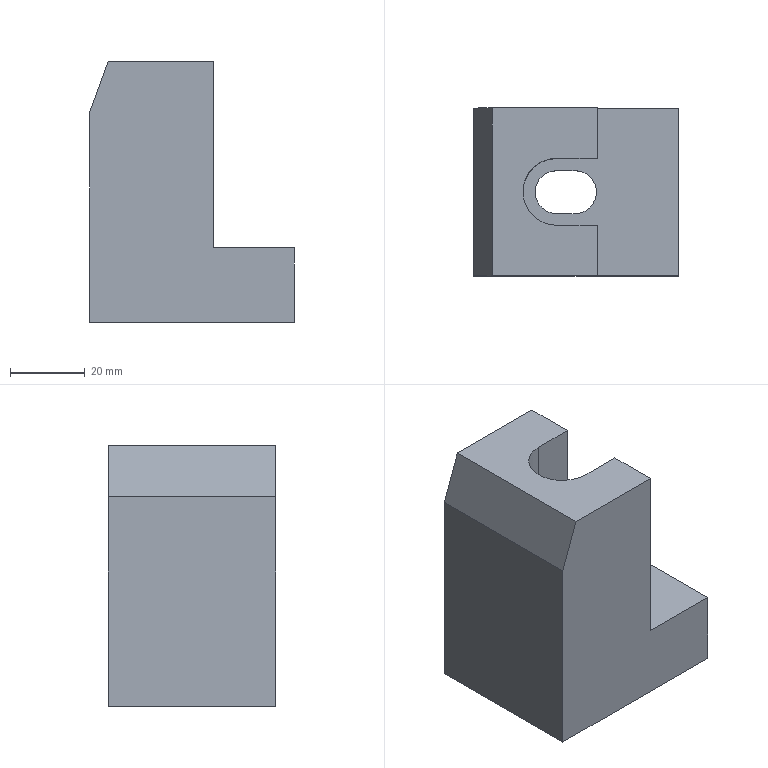Part | STEP file | lll_id5026_x_t | 1 solid | 17 faces | box 55 x 45 x 70 mm | volume 103267 mm3 | plane 14 | cylinder 3 | commonest cylinder face diameters 11.509 x2 18.008 x1
STEP:
#1=CARTESIAN_POINT('',(2858.213,-91.496,0.));
#2=VERTEX_POINT('',#1);
#3=CARTESIAN_POINT('',(2858.213,-78.,0.));
#4=VERTEX_POINT('',#3);
#5=CARTESIAN_POINT('',(2858.213,-123.,0.));
#6=DIRECTION('',(0.,1.,0.));
#7=VECTOR('',#6,1.);
#8=LINE('',#5,#7);
#9=EDGE_CURVE('',#2,#4,#8,.T.);
#10=ORIENTED_EDGE('',*,*,#9,.T.);
#11=CARTESIAN_POINT('',(2858.213,-78.,50.));
#12=VERTEX_POINT('',#11);
#13=CARTESIAN_POINT('',(2858.213,-78.,25.));
#14=DIRECTION('',(0.,0.,-1.));
#15=VECTOR('',#14,1.);
#16=LINE('',#13,#15);
#17=EDGE_CURVE('',#12,#4,#16,.T.);
#18=ORIENTED_EDGE('',*,*,#17,.F.);
#19=CARTESIAN_POINT('',(2858.213,-91.496,50.));
#20=VERTEX_POINT('',#19);
#21=CARTESIAN_POINT('',(2858.213,-173.,50.));
#22=DIRECTION('',(0.,1.,0.));
#23=VECTOR('',#22,1.);
#24=LINE('',#21,#23);
#25=EDGE_CURVE('',#20,#12,#24,.T.);
#26=ORIENTED_EDGE('',*,*,#25,.F.);
#27=CARTESIAN_POINT('',(2858.213,-91.496,0.));
#28=DIRECTION('',(0.,0.,1.));
#29=VECTOR('',#28,1.);
#30=LINE('',#27,#29);
#31=EDGE_CURVE('',#2,#20,#30,.T.);
#32=ORIENTED_EDGE('',*,*,#31,.F.);
#33=EDGE_LOOP('',(#10,#18,#26,#32));
#34=FACE_OUTER_BOUND('',#33,.T.);
#35=CARTESIAN_POINT('',(2858.213,-173.,50.));
#36=DIRECTION('',(1.,0.,0.));
#37=DIRECTION('',(0.,0.,1.));
#38=AXIS2_PLACEMENT_3D('',#35,#36,#37);
#39=PLANE('',#38);
#40=ADVANCED_FACE('',(#34),#39,.T.);
#41=CARTESIAN_POINT('',(2824.963,-78.,-20.));
#42=VERTEX_POINT('',#41);
#43=CARTESIAN_POINT('',(2824.963,-78.,36.263));
#44=VERTEX_POINT('',#43);
#45=CARTESIAN_POINT('',(2824.963,-78.,50.));
#46=DIRECTION('',(0.,0.,1.));
#47=VECTOR('',#46,1.);
#48=LINE('',#45,#47);
#49=EDGE_CURVE('',#42,#44,#48,.T.);
#50=ORIENTED_EDGE('',*,*,#49,.F.);
#51=CARTESIAN_POINT('',(2824.963,-123.,-20.));
#52=VERTEX_POINT('',#51);
#53=CARTESIAN_POINT('',(2824.963,-88.5,-20.));
#54=DIRECTION('',(0.,1.,0.));
#55=VECTOR('',#54,1.);
#56=LINE('',#53,#55);
#57=EDGE_CURVE('',#52,#42,#56,.T.);
#58=ORIENTED_EDGE('',*,*,#57,.F.);
#59=CARTESIAN_POINT('',(2824.963,-123.,36.263));
#60=VERTEX_POINT('',#59);
#61=CARTESIAN_POINT('',(2824.963,-123.,50.));
#62=DIRECTION('',(0.,0.,-1.));
#63=VECTOR('',#62,1.);
#64=LINE('',#61,#63);
#65=EDGE_CURVE('',#60,#52,#64,.T.);
#66=ORIENTED_EDGE('',*,*,#65,.F.);
#67=CARTESIAN_POINT('',(2824.963,-88.5,36.263));
#68=DIRECTION('',(0.,-1.,0.));
#69=VECTOR('',#68,1.);
#70=LINE('',#67,#69);
#71=EDGE_CURVE('',#44,#60,#70,.T.);
#72=ORIENTED_EDGE('',*,*,#71,.F.);
#73=EDGE_LOOP('',(#50,#58,#66,#72));
#74=FACE_OUTER_BOUND('',#73,.T.);
#75=CARTESIAN_POINT('',(2824.963,-173.,50.));
#76=DIRECTION('',(1.,0.,0.));
#77=DIRECTION('',(0.,0.,1.));
#78=AXIS2_PLACEMENT_3D('',#75,#76,#77);
#79=PLANE('',#78);
#80=ADVANCED_FACE('',(#74),#79,.F.);
#81=CARTESIAN_POINT('',(2879.963,-123.,0.));
#82=VERTEX_POINT('',#81);
#83=CARTESIAN_POINT('',(2858.213,-123.,0.));
#84=VERTEX_POINT('',#83);
#85=CARTESIAN_POINT('',(2873.213,-123.,0.));
#86=DIRECTION('',(-1.,0.,0.));
#87=VECTOR('',#86,1.);
#88=LINE('',#85,#87);
#89=EDGE_CURVE('',#82,#84,#88,.T.);
#90=ORIENTED_EDGE('',*,*,#89,.T.);
#91=CARTESIAN_POINT('',(2858.213,-123.,50.));
#92=VERTEX_POINT('',#91);
#93=CARTESIAN_POINT('',(2858.213,-123.,50.));
#94=DIRECTION('',(0.,0.,-1.));
#95=VECTOR('',#94,1.);
#96=LINE('',#93,#95);
#97=EDGE_CURVE('',#92,#84,#96,.T.);
#98=ORIENTED_EDGE('',*,*,#97,.F.);
#99=CARTESIAN_POINT('',(2829.963,-123.,50.));
#100=VERTEX_POINT('',#99);
#101=CARTESIAN_POINT('',(2839.963,-123.,50.));
#102=DIRECTION('',(-1.,0.,0.));
#103=VECTOR('',#102,1.);
#104=LINE('',#101,#103);
#105=EDGE_CURVE('',#92,#100,#104,.T.);
#106=ORIENTED_EDGE('',*,*,#105,.T.);
#107=CARTESIAN_POINT('',(2829.963,-123.,50.));
#108=DIRECTION('',(0.342,0.,0.9397));
#109=VECTOR('',#108,1.);
#110=LINE('',#107,#109);
#111=EDGE_CURVE('',#60,#100,#110,.T.);
#112=ORIENTED_EDGE('',*,*,#111,.F.);
#113=ORIENTED_EDGE('',*,*,#65,.T.);
#114=CARTESIAN_POINT('',(2879.963,-123.,-20.));
#115=VERTEX_POINT('',#114);
#116=CARTESIAN_POINT('',(2839.963,-123.,-20.));
#117=DIRECTION('',(-1.,0.,0.));
#118=VECTOR('',#117,1.);
#119=LINE('',#116,#118);
#120=EDGE_CURVE('',#115,#52,#119,.T.);
#121=ORIENTED_EDGE('',*,*,#120,.F.);
#122=CARTESIAN_POINT('',(2879.963,-123.,50.));
#123=DIRECTION('',(0.,0.,-1.));
#124=VECTOR('',#123,1.);
#125=LINE('',#122,#124);
#126=EDGE_CURVE('',#82,#115,#125,.T.);
#127=ORIENTED_EDGE('',*,*,#126,.F.);
#128=EDGE_LOOP('',(#90,#98,#106,#112,#113,#121,#127));
#129=FACE_OUTER_BOUND('',#128,.T.);
#130=CARTESIAN_POINT('',(2858.213,-123.,50.));
#131=DIRECTION('',(0.,1.,0.));
#132=DIRECTION('',(0.,0.,1.));
#133=AXIS2_PLACEMENT_3D('',#130,#131,#132);
#134=PLANE('',#133);
#135=ADVANCED_FACE('',(#129),#134,.F.);
#136=CARTESIAN_POINT('',(2858.213,-109.504,50.));
#137=VERTEX_POINT('',#136);
#138=CARTESIAN_POINT('',(2858.213,-173.,50.));
#139=DIRECTION('',(0.,1.,0.));
#140=VECTOR('',#139,1.);
#141=LINE('',#138,#140);
#142=EDGE_CURVE('',#92,#137,#141,.T.);
#143=ORIENTED_EDGE('',*,*,#142,.F.);
#144=ORIENTED_EDGE('',*,*,#97,.T.);
#145=CARTESIAN_POINT('',(2858.213,-109.504,0.));
#146=VERTEX_POINT('',#145);
#147=CARTESIAN_POINT('',(2858.213,-123.,0.));
#148=DIRECTION('',(0.,1.,0.));
#149=VECTOR('',#148,1.);
#150=LINE('',#147,#149);
#151=EDGE_CURVE('',#84,#146,#150,.T.);
#152=ORIENTED_EDGE('',*,*,#151,.T.);
#153=CARTESIAN_POINT('',(2858.213,-109.504,113.));
#154=DIRECTION('',(0.,0.,-1.));
#155=VECTOR('',#154,1.);
#156=LINE('',#153,#155);
#157=EDGE_CURVE('',#137,#146,#156,.T.);
#158=ORIENTED_EDGE('',*,*,#157,.F.);
#159=EDGE_LOOP('',(#143,#144,#152,#158));
#160=FACE_OUTER_BOUND('',#159,.T.);
#161=CARTESIAN_POINT('',(2858.213,-173.,50.));
#162=DIRECTION('',(1.,0.,0.));
#163=DIRECTION('',(0.,0.,1.));
#164=AXIS2_PLACEMENT_3D('',#161,#162,#163);
#165=PLANE('',#164);
#166=ADVANCED_FACE('',(#160),#165,.T.);
#167=CARTESIAN_POINT('',(2879.963,-78.,-20.));
#168=VERTEX_POINT('',#167);
#169=CARTESIAN_POINT('',(2839.963,-78.,-20.));
#170=DIRECTION('',(1.,0.,0.));
#171=VECTOR('',#170,1.);
#172=LINE('',#169,#171);
#173=EDGE_CURVE('',#42,#168,#172,.T.);
#174=ORIENTED_EDGE('',*,*,#173,.F.);
#175=ORIENTED_EDGE('',*,*,#49,.T.);
#176=CARTESIAN_POINT('',(2829.963,-78.,50.));
#177=VERTEX_POINT('',#176);
#178=CARTESIAN_POINT('',(2829.963,-78.,50.));
#179=DIRECTION('',(-0.342,0.,-0.9397));
#180=VECTOR('',#179,1.);
#181=LINE('',#178,#180);
#182=EDGE_CURVE('',#177,#44,#181,.T.);
#183=ORIENTED_EDGE('',*,*,#182,.F.);
#184=CARTESIAN_POINT('',(2841.588,-78.,50.));
#185=DIRECTION('',(-1.,0.,0.));
#186=VECTOR('',#185,1.);
#187=LINE('',#184,#186);
#188=EDGE_CURVE('',#12,#177,#187,.T.);
#189=ORIENTED_EDGE('',*,*,#188,.F.);
#190=ORIENTED_EDGE('',*,*,#17,.T.);
#191=CARTESIAN_POINT('',(2879.963,-78.,0.));
#192=VERTEX_POINT('',#191);
#193=CARTESIAN_POINT('',(2841.588,-78.,0.));
#194=DIRECTION('',(-1.,0.,0.));
#195=VECTOR('',#194,1.);
#196=LINE('',#193,#195);
#197=EDGE_CURVE('',#192,#4,#196,.T.);
#198=ORIENTED_EDGE('',*,*,#197,.F.);
#199=CARTESIAN_POINT('',(2879.963,-78.,25.));
#200=DIRECTION('',(0.,0.,1.));
#201=VECTOR('',#200,1.);
#202=LINE('',#199,#201);
#203=EDGE_CURVE('',#168,#192,#202,.T.);
#204=ORIENTED_EDGE('',*,*,#203,.F.);
#205=EDGE_LOOP('',(#174,#175,#183,#189,#190,#198,#204));
#206=FACE_OUTER_BOUND('',#205,.T.);
#207=CARTESIAN_POINT('',(2841.588,-78.,25.));
#208=DIRECTION('',(0.,-1.,0.));
#209=DIRECTION('',(0.,0.,-1.));
#210=AXIS2_PLACEMENT_3D('',#207,#208,#209);
#211=PLANE('',#210);
#212=ADVANCED_FACE('',(#206),#211,.F.);
#213=CARTESIAN_POINT('',(2879.963,-88.5,-20.));
#214=DIRECTION('',(0.,1.,0.));
#215=VECTOR('',#214,1.);
#216=LINE('',#213,#215);
#217=EDGE_CURVE('',#115,#168,#216,.T.);
#218=ORIENTED_EDGE('',*,*,#217,.F.);
#219=ORIENTED_EDGE('',*,*,#120,.T.);
#220=ORIENTED_EDGE('',*,*,#57,.T.);
#221=ORIENTED_EDGE('',*,*,#173,.T.);
#222=EDGE_LOOP('',(#218,#219,#220,#221));
#223=FACE_BOUND('',#222,.T.);
#224=CARTESIAN_POINT('',(2847.217,-94.745,-20.));
#225=VERTEX_POINT('',#224);
#226=CARTESIAN_POINT('',(2847.217,-106.254,-20.));
#227=VERTEX_POINT('',#226);
#228=CARTESIAN_POINT('',(2847.217,-100.5,-20.));
#229=DIRECTION('',(0.,0.,1.));
#230=DIRECTION('',(1.,0.,0.));
#231=AXIS2_PLACEMENT_3D('',#228,#229,#230);
#232=CIRCLE('',#231,5.755);
#233=EDGE_CURVE('',#225,#227,#232,.T.);
#234=ORIENTED_EDGE('',*,*,#233,.T.);
#235=CARTESIAN_POINT('',(2852.217,-106.254,-20.));
#236=VERTEX_POINT('',#235);
#237=CARTESIAN_POINT('',(2839.963,-106.254,-20.));
#238=DIRECTION('',(-1.,0.,0.));
#239=VECTOR('',#238,1.);
#240=LINE('',#237,#239);
#241=EDGE_CURVE('',#236,#227,#240,.T.);
#242=ORIENTED_EDGE('',*,*,#241,.F.);
#243=CARTESIAN_POINT('',(2852.217,-94.745,-20.));
#244=VERTEX_POINT('',#243);
#245=CARTESIAN_POINT('',(2852.217,-100.5,-20.));
#246=DIRECTION('',(0.,0.,1.));
#247=DIRECTION('',(1.,0.,0.));
#248=AXIS2_PLACEMENT_3D('',#245,#246,#247);
#249=CIRCLE('',#248,5.755);
#250=EDGE_CURVE('',#236,#244,#249,.T.);
#251=ORIENTED_EDGE('',*,*,#250,.T.);
#252=CARTESIAN_POINT('',(2839.963,-94.745,-20.));
#253=DIRECTION('',(1.,0.,0.));
#254=VECTOR('',#253,1.);
#255=LINE('',#252,#254);
#256=EDGE_CURVE('',#225,#244,#255,.T.);
#257=ORIENTED_EDGE('',*,*,#256,.F.);
#258=EDGE_LOOP('',(#234,#242,#251,#257));
#259=FACE_BOUND('',#258,.T.);
#260=CARTESIAN_POINT('',(2839.963,-88.5,-20.));
#261=DIRECTION('',(0.,0.,-1.));
#262=DIRECTION('',(1.,0.,0.));
#263=AXIS2_PLACEMENT_3D('',#260,#261,#262);
#264=PLANE('',#263);
#265=ADVANCED_FACE('',(#223,#259),#264,.T.);
#266=CARTESIAN_POINT('',(2847.217,-109.504,50.));
#267=VERTEX_POINT('',#266);
#268=CARTESIAN_POINT('',(2839.963,-109.504,50.));
#269=DIRECTION('',(1.,0.,0.));
#270=VECTOR('',#269,1.);
#271=LINE('',#268,#270);
#272=EDGE_CURVE('',#267,#137,#271,.T.);
#273=ORIENTED_EDGE('',*,*,#272,.F.);
#274=CARTESIAN_POINT('',(2847.217,-91.496,50.));
#275=VERTEX_POINT('',#274);
#276=CARTESIAN_POINT('',(2847.217,-100.5,50.));
#277=DIRECTION('',(0.,0.,1.));
#278=DIRECTION('',(1.,0.,0.));
#279=AXIS2_PLACEMENT_3D('',#276,#277,#278);
#280=CIRCLE('',#279,9.004);
#281=EDGE_CURVE('',#275,#267,#280,.T.);
#282=ORIENTED_EDGE('',*,*,#281,.F.);
#283=CARTESIAN_POINT('',(2839.963,-91.496,50.));
#284=DIRECTION('',(-1.,0.,0.));
#285=VECTOR('',#284,1.);
#286=LINE('',#283,#285);
#287=EDGE_CURVE('',#20,#275,#286,.T.);
#288=ORIENTED_EDGE('',*,*,#287,.F.);
#289=ORIENTED_EDGE('',*,*,#25,.T.);
#290=ORIENTED_EDGE('',*,*,#188,.T.);
#291=CARTESIAN_POINT('',(2829.963,-88.5,50.));
#292=DIRECTION('',(0.,1.,0.));
#293=VECTOR('',#292,1.);
#294=LINE('',#291,#293);
#295=EDGE_CURVE('',#100,#177,#294,.T.);
#296=ORIENTED_EDGE('',*,*,#295,.F.);
#297=ORIENTED_EDGE('',*,*,#105,.F.);
#298=ORIENTED_EDGE('',*,*,#142,.T.);
#299=EDGE_LOOP('',(#273,#282,#288,#289,#290,#296,#297,#298));
#300=FACE_OUTER_BOUND('',#299,.T.);
#301=CARTESIAN_POINT('',(2839.963,-88.5,50.));
#302=DIRECTION('',(0.,0.,-1.));
#303=DIRECTION('',(1.,0.,0.));
#304=AXIS2_PLACEMENT_3D('',#301,#302,#303);
#305=PLANE('',#304);
#306=ADVANCED_FACE('',(#300),#305,.F.);
#307=ORIENTED_EDGE('',*,*,#111,.T.);
#308=ORIENTED_EDGE('',*,*,#295,.T.);
#309=ORIENTED_EDGE('',*,*,#182,.T.);
#310=ORIENTED_EDGE('',*,*,#71,.T.);
#311=EDGE_LOOP('',(#307,#308,#309,#310));
#312=FACE_OUTER_BOUND('',#311,.T.);
#313=CARTESIAN_POINT('',(2829.963,-88.5,50.));
#314=DIRECTION('',(0.9397,0.,-0.342));
#315=DIRECTION('',(0.342,0.,0.9397));
#316=AXIS2_PLACEMENT_3D('',#313,#314,#315);
#317=PLANE('',#316);
#318=ADVANCED_FACE('',(#312),#317,.F.);
#319=ORIENTED_EDGE('',*,*,#197,.T.);
#320=ORIENTED_EDGE('',*,*,#9,.F.);
#321=CARTESIAN_POINT('',(2847.217,-91.496,0.));
#322=VERTEX_POINT('',#321);
#323=CARTESIAN_POINT('',(2852.217,-91.496,0.));
#324=DIRECTION('',(-1.,0.,0.));
#325=VECTOR('',#324,1.);
#326=LINE('',#323,#325);
#327=EDGE_CURVE('',#2,#322,#326,.T.);
#328=ORIENTED_EDGE('',*,*,#327,.T.);
#329=CARTESIAN_POINT('',(2847.217,-109.504,0.));
#330=VERTEX_POINT('',#329);
#331=CARTESIAN_POINT('',(2847.217,-100.5,0.));
#332=DIRECTION('',(0.,0.,-1.));
#333=DIRECTION('',(-1.,0.,0.));
#334=AXIS2_PLACEMENT_3D('',#331,#332,#333);
#335=CIRCLE('',#334,9.004);
#336=EDGE_CURVE('',#330,#322,#335,.T.);
#337=ORIENTED_EDGE('',*,*,#336,.F.);
#338=CARTESIAN_POINT('',(2852.217,-109.504,0.));
#339=DIRECTION('',(-1.,0.,0.));
#340=VECTOR('',#339,1.);
#341=LINE('',#338,#340);
#342=EDGE_CURVE('',#146,#330,#341,.T.);
#343=ORIENTED_EDGE('',*,*,#342,.F.);
#344=ORIENTED_EDGE('',*,*,#151,.F.);
#345=ORIENTED_EDGE('',*,*,#89,.F.);
#346=CARTESIAN_POINT('',(2879.963,-123.,0.));
#347=DIRECTION('',(0.,-1.,0.));
#348=VECTOR('',#347,1.);
#349=LINE('',#346,#348);
#350=EDGE_CURVE('',#192,#82,#349,.T.);
#351=ORIENTED_EDGE('',*,*,#350,.F.);
#352=EDGE_LOOP('',(#319,#320,#328,#337,#343,#344,#345,#351));
#353=FACE_BOUND('',#352,.T.);
#354=CARTESIAN_POINT('',(2852.217,-106.254,0.));
#355=VERTEX_POINT('',#354);
#356=CARTESIAN_POINT('',(2847.217,-106.254,0.));
#357=VERTEX_POINT('',#356);
#358=CARTESIAN_POINT('',(2852.217,-106.254,0.));
#359=DIRECTION('',(-1.,0.,0.));
#360=VECTOR('',#359,1.);
#361=LINE('',#358,#360);
#362=EDGE_CURVE('',#355,#357,#361,.T.);
#363=ORIENTED_EDGE('',*,*,#362,.T.);
#364=CARTESIAN_POINT('',(2847.217,-94.745,0.));
#365=VERTEX_POINT('',#364);
#366=CARTESIAN_POINT('',(2847.217,-100.5,0.));
#367=DIRECTION('',(0.,0.,-1.));
#368=DIRECTION('',(1.,0.,0.));
#369=AXIS2_PLACEMENT_3D('',#366,#367,#368);
#370=CIRCLE('',#369,5.755);
#371=EDGE_CURVE('',#357,#365,#370,.T.);
#372=ORIENTED_EDGE('',*,*,#371,.T.);
#373=CARTESIAN_POINT('',(2852.217,-94.745,0.));
#374=VERTEX_POINT('',#373);
#375=CARTESIAN_POINT('',(2852.217,-94.745,0.));
#376=DIRECTION('',(-1.,0.,0.));
#377=VECTOR('',#376,1.);
#378=LINE('',#375,#377);
#379=EDGE_CURVE('',#374,#365,#378,.T.);
#380=ORIENTED_EDGE('',*,*,#379,.F.);
#381=CARTESIAN_POINT('',(2852.217,-100.5,0.));
#382=DIRECTION('',(0.,0.,-1.));
#383=DIRECTION('',(1.,0.,0.));
#384=AXIS2_PLACEMENT_3D('',#381,#382,#383);
#385=CIRCLE('',#384,5.755);
#386=EDGE_CURVE('',#374,#355,#385,.T.);
#387=ORIENTED_EDGE('',*,*,#386,.T.);
#388=EDGE_LOOP('',(#363,#372,#380,#387));
#389=FACE_BOUND('',#388,.T.);
#390=CARTESIAN_POINT('',(2873.213,-123.,0.));
#391=DIRECTION('',(0.,0.,-1.));
#392=DIRECTION('',(1.,0.,0.));
#393=AXIS2_PLACEMENT_3D('',#390,#391,#392);
#394=PLANE('',#393);
#395=ADVANCED_FACE('',(#353,#389),#394,.F.);
#396=CARTESIAN_POINT('',(2847.217,-91.496,13.));
#397=DIRECTION('',(0.,0.,-1.));
#398=VECTOR('',#397,1.);
#399=LINE('',#396,#398);
#400=EDGE_CURVE('',#275,#322,#399,.T.);
#401=ORIENTED_EDGE('',*,*,#400,.F.);
#402=ORIENTED_EDGE('',*,*,#281,.T.);
#403=CARTESIAN_POINT('',(2847.217,-109.504,13.));
#404=DIRECTION('',(0.,0.,1.));
#405=VECTOR('',#404,1.);
#406=LINE('',#403,#405);
#407=EDGE_CURVE('',#330,#267,#406,.T.);
#408=ORIENTED_EDGE('',*,*,#407,.F.);
#409=ORIENTED_EDGE('',*,*,#336,.T.);
#410=EDGE_LOOP('',(#401,#402,#408,#409));
#411=FACE_OUTER_BOUND('',#410,.T.);
#412=CARTESIAN_POINT('',(2847.217,-100.5,13.));
#413=DIRECTION('',(0.,0.,-1.));
#414=DIRECTION('',(-1.,0.,0.));
#415=AXIS2_PLACEMENT_3D('',#412,#413,#414);
#416=CYLINDRICAL_SURFACE('',#415,9.004);
#417=ADVANCED_FACE('',(#411),#416,.F.);
#418=ORIENTED_EDGE('',*,*,#407,.T.);
#419=ORIENTED_EDGE('',*,*,#272,.T.);
#420=ORIENTED_EDGE('',*,*,#157,.T.);
#421=ORIENTED_EDGE('',*,*,#342,.T.);
#422=EDGE_LOOP('',(#418,#419,#420,#421));
#423=FACE_OUTER_BOUND('',#422,.T.);
#424=CARTESIAN_POINT('',(2852.217,-109.504,113.));
#425=DIRECTION('',(0.,-1.,0.));
#426=DIRECTION('',(0.,0.,-1.));
#427=AXIS2_PLACEMENT_3D('',#424,#425,#426);
#428=PLANE('',#427);
#429=ADVANCED_FACE('',(#423),#428,.F.);
#430=ORIENTED_EDGE('',*,*,#287,.T.);
#431=ORIENTED_EDGE('',*,*,#400,.T.);
#432=ORIENTED_EDGE('',*,*,#327,.F.);
#433=ORIENTED_EDGE('',*,*,#31,.T.);
#434=EDGE_LOOP('',(#430,#431,#432,#433));
#435=FACE_OUTER_BOUND('',#434,.T.);
#436=CARTESIAN_POINT('',(2852.217,-91.496,0.));
#437=DIRECTION('',(0.,1.,0.));
#438=DIRECTION('',(0.,0.,1.));
#439=AXIS2_PLACEMENT_3D('',#436,#437,#438);
#440=PLANE('',#439);
#441=ADVANCED_FACE('',(#435),#440,.F.);
#442=ORIENTED_EDGE('',*,*,#233,.F.);
#443=CARTESIAN_POINT('',(2847.217,-94.745,13.));
#444=DIRECTION('',(0.,0.,1.));
#445=VECTOR('',#444,1.);
#446=LINE('',#443,#445);
#447=EDGE_CURVE('',#225,#365,#446,.T.);
#448=ORIENTED_EDGE('',*,*,#447,.T.);
#449=ORIENTED_EDGE('',*,*,#371,.F.);
#450=CARTESIAN_POINT('',(2847.217,-106.254,13.));
#451=DIRECTION('',(0.,0.,-1.));
#452=VECTOR('',#451,1.);
#453=LINE('',#450,#452);
#454=EDGE_CURVE('',#357,#227,#453,.T.);
#455=ORIENTED_EDGE('',*,*,#454,.T.);
#456=EDGE_LOOP('',(#442,#448,#449,#455));
#457=FACE_OUTER_BOUND('',#456,.T.);
#458=CARTESIAN_POINT('',(2847.217,-100.5,13.));
#459=DIRECTION('',(0.,0.,-1.));
#460=DIRECTION('',(-1.,0.,0.));
#461=AXIS2_PLACEMENT_3D('',#458,#459,#460);
#462=CYLINDRICAL_SURFACE('',#461,5.755);
#463=ADVANCED_FACE('',(#457),#462,.F.);
#464=CARTESIAN_POINT('',(2852.217,-106.254,-57.));
#465=DIRECTION('',(0.,0.,-1.));
#466=VECTOR('',#465,1.);
#467=LINE('',#464,#466);
#468=EDGE_CURVE('',#355,#236,#467,.T.);
#469=ORIENTED_EDGE('',*,*,#468,.T.);
#470=ORIENTED_EDGE('',*,*,#241,.T.);
#471=ORIENTED_EDGE('',*,*,#454,.F.);
#472=ORIENTED_EDGE('',*,*,#362,.F.);
#473=EDGE_LOOP('',(#469,#470,#471,#472));
#474=FACE_OUTER_BOUND('',#473,.T.);
#475=CARTESIAN_POINT('',(2852.217,-106.254,-57.));
#476=DIRECTION('',(0.,1.,0.));
#477=DIRECTION('',(0.,0.,1.));
#478=AXIS2_PLACEMENT_3D('',#475,#476,#477);
#479=PLANE('',#478);
#480=ADVANCED_FACE('',(#474),#479,.T.);
#481=ORIENTED_EDGE('',*,*,#447,.F.);
#482=ORIENTED_EDGE('',*,*,#256,.T.);
#483=CARTESIAN_POINT('',(2852.217,-94.745,0.));
#484=DIRECTION('',(0.,0.,1.));
#485=VECTOR('',#484,1.);
#486=LINE('',#483,#485);
#487=EDGE_CURVE('',#244,#374,#486,.T.);
#488=ORIENTED_EDGE('',*,*,#487,.T.);
#489=ORIENTED_EDGE('',*,*,#379,.T.);
#490=EDGE_LOOP('',(#481,#482,#488,#489));
#491=FACE_OUTER_BOUND('',#490,.T.);
#492=CARTESIAN_POINT('',(2852.217,-94.745,0.));
#493=DIRECTION('',(0.,-1.,0.));
#494=DIRECTION('',(0.,0.,-1.));
#495=AXIS2_PLACEMENT_3D('',#492,#493,#494);
#496=PLANE('',#495);
#497=ADVANCED_FACE('',(#491),#496,.T.);
#498=ORIENTED_EDGE('',*,*,#250,.F.);
#499=ORIENTED_EDGE('',*,*,#468,.F.);
#500=ORIENTED_EDGE('',*,*,#386,.F.);
#501=ORIENTED_EDGE('',*,*,#487,.F.);
#502=EDGE_LOOP('',(#498,#499,#500,#501));
#503=FACE_OUTER_BOUND('',#502,.T.);
#504=CARTESIAN_POINT('',(2852.217,-100.5,13.));
#505=DIRECTION('',(0.,0.,-1.));
#506=DIRECTION('',(-1.,0.,0.));
#507=AXIS2_PLACEMENT_3D('',#504,#505,#506);
#508=CYLINDRICAL_SURFACE('',#507,5.755);
#509=ADVANCED_FACE('',(#503),#508,.F.);
#510=ORIENTED_EDGE('',*,*,#217,.T.);
#511=ORIENTED_EDGE('',*,*,#203,.T.);
#512=ORIENTED_EDGE('',*,*,#350,.T.);
#513=ORIENTED_EDGE('',*,*,#126,.T.);
#514=EDGE_LOOP('',(#510,#511,#512,#513));
#515=FACE_OUTER_BOUND('',#514,.T.);
#516=CARTESIAN_POINT('',(2879.963,-100.5,8.131));
#517=DIRECTION('',(-1.,0.,0.));
#518=DIRECTION('',(0.,0.,-1.));
#519=AXIS2_PLACEMENT_3D('',#516,#517,#518);
#520=PLANE('',#519);
#521=ADVANCED_FACE('',(#515),#520,.F.);
#522=CLOSED_SHELL('',(#40,#80,#135,#166,#212,#265,#306,#318,#395,#417,#429,#441,#463,#480,#497,#509,#521));
#523=MANIFOLD_SOLID_BREP('',#522);
#524=(LENGTH_UNIT()NAMED_UNIT(*)SI_UNIT(.MILLI.,.METRE.));
#525=UNCERTAINTY_MEASURE_WITH_UNIT(LENGTH_MEASURE(0.00002),#524,'','');
#526=(NAMED_UNIT(*)PLANE_ANGLE_UNIT()SI_UNIT($,.RADIAN.));
#527=PLANE_ANGLE_MEASURE_WITH_UNIT(PLANE_ANGLE_MEASURE(0.01745),#526);
#528=DIMENSIONAL_EXPONENTS(0.,0.,0.,0.,0.,0.,0.);
#529=(CONVERSION_BASED_UNIT('DEGREE',#527)NAMED_UNIT(#528)PLANE_ANGLE_UNIT());
#530=(NAMED_UNIT(*)SI_UNIT($,.STERADIAN.)SOLID_ANGLE_UNIT());
#531=(GEOMETRIC_REPRESENTATION_CONTEXT(3)GLOBAL_UNCERTAINTY_ASSIGNED_CONTEXT((#525))GLOBAL_UNIT_ASSIGNED_CONTEXT((#524,#529,#530))REPRESENTATION_CONTEXT('',''));
#532=ADVANCED_BREP_SHAPE_REPRESENTATION('',(#523),#531);